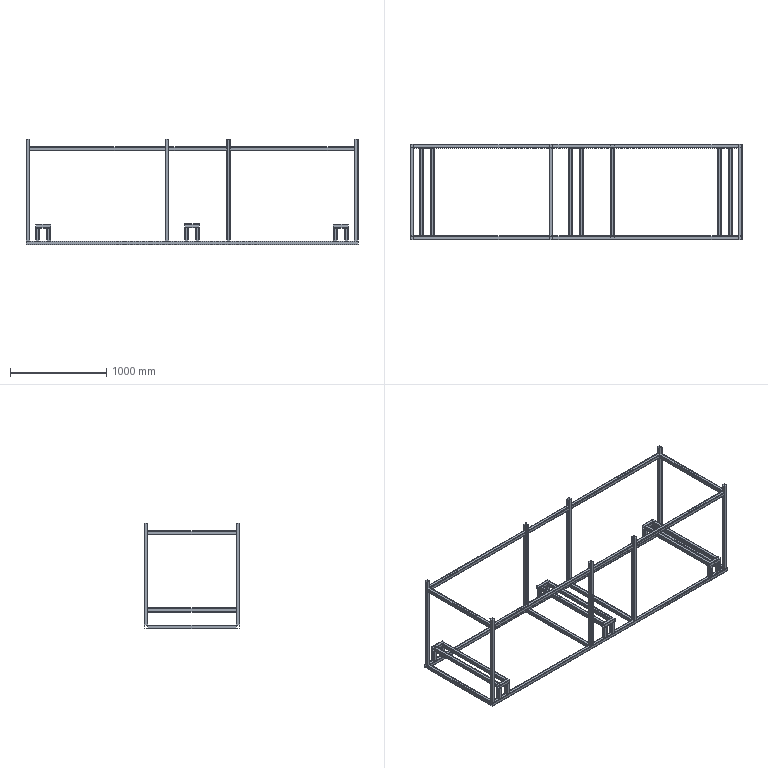Part | SolidWorks | features WeldCornerFeat 8, 3DProfileFeature 1, MirrorSolid 1, WeldMemberFeat 1, WeldmentFeature 1 | 46 solids | 828 faces | box 3455 x 996 x 1100 mm | volume 14945108 mm3 | plane 460 | cylinder 368 | commonest cylinder face diameters 6 x184 12 x184